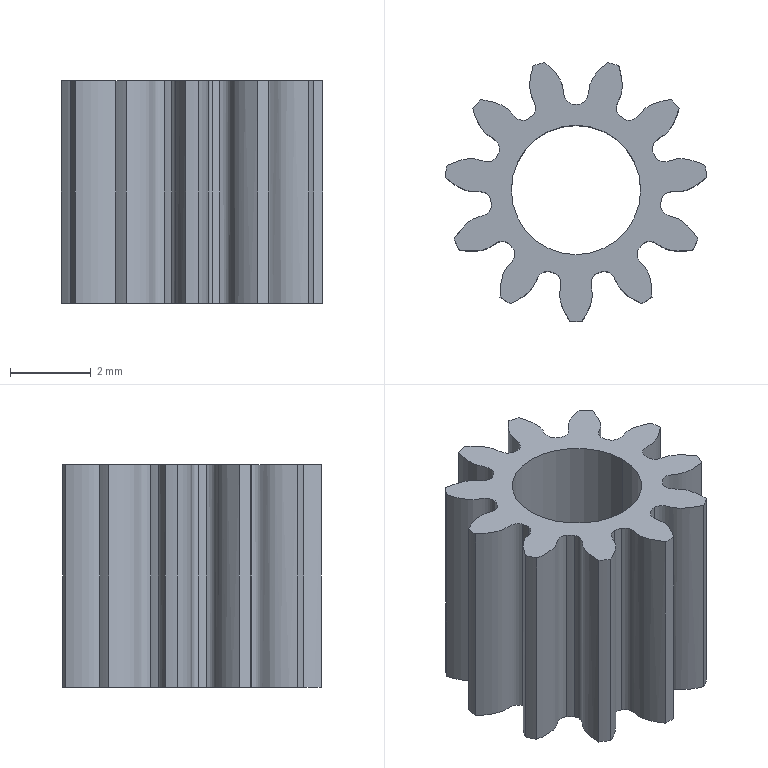Part | SolidWorks | features BaseBody 1 | 1 solid | 48 faces | box 6.47 x 6.407 x 5.5 mm | volume 81.586 mm3 | cylinder 24 | spline 22 | plane 2 | commonest cylinder face diameters 4.25 x11 6.5 x11 3.2 x2